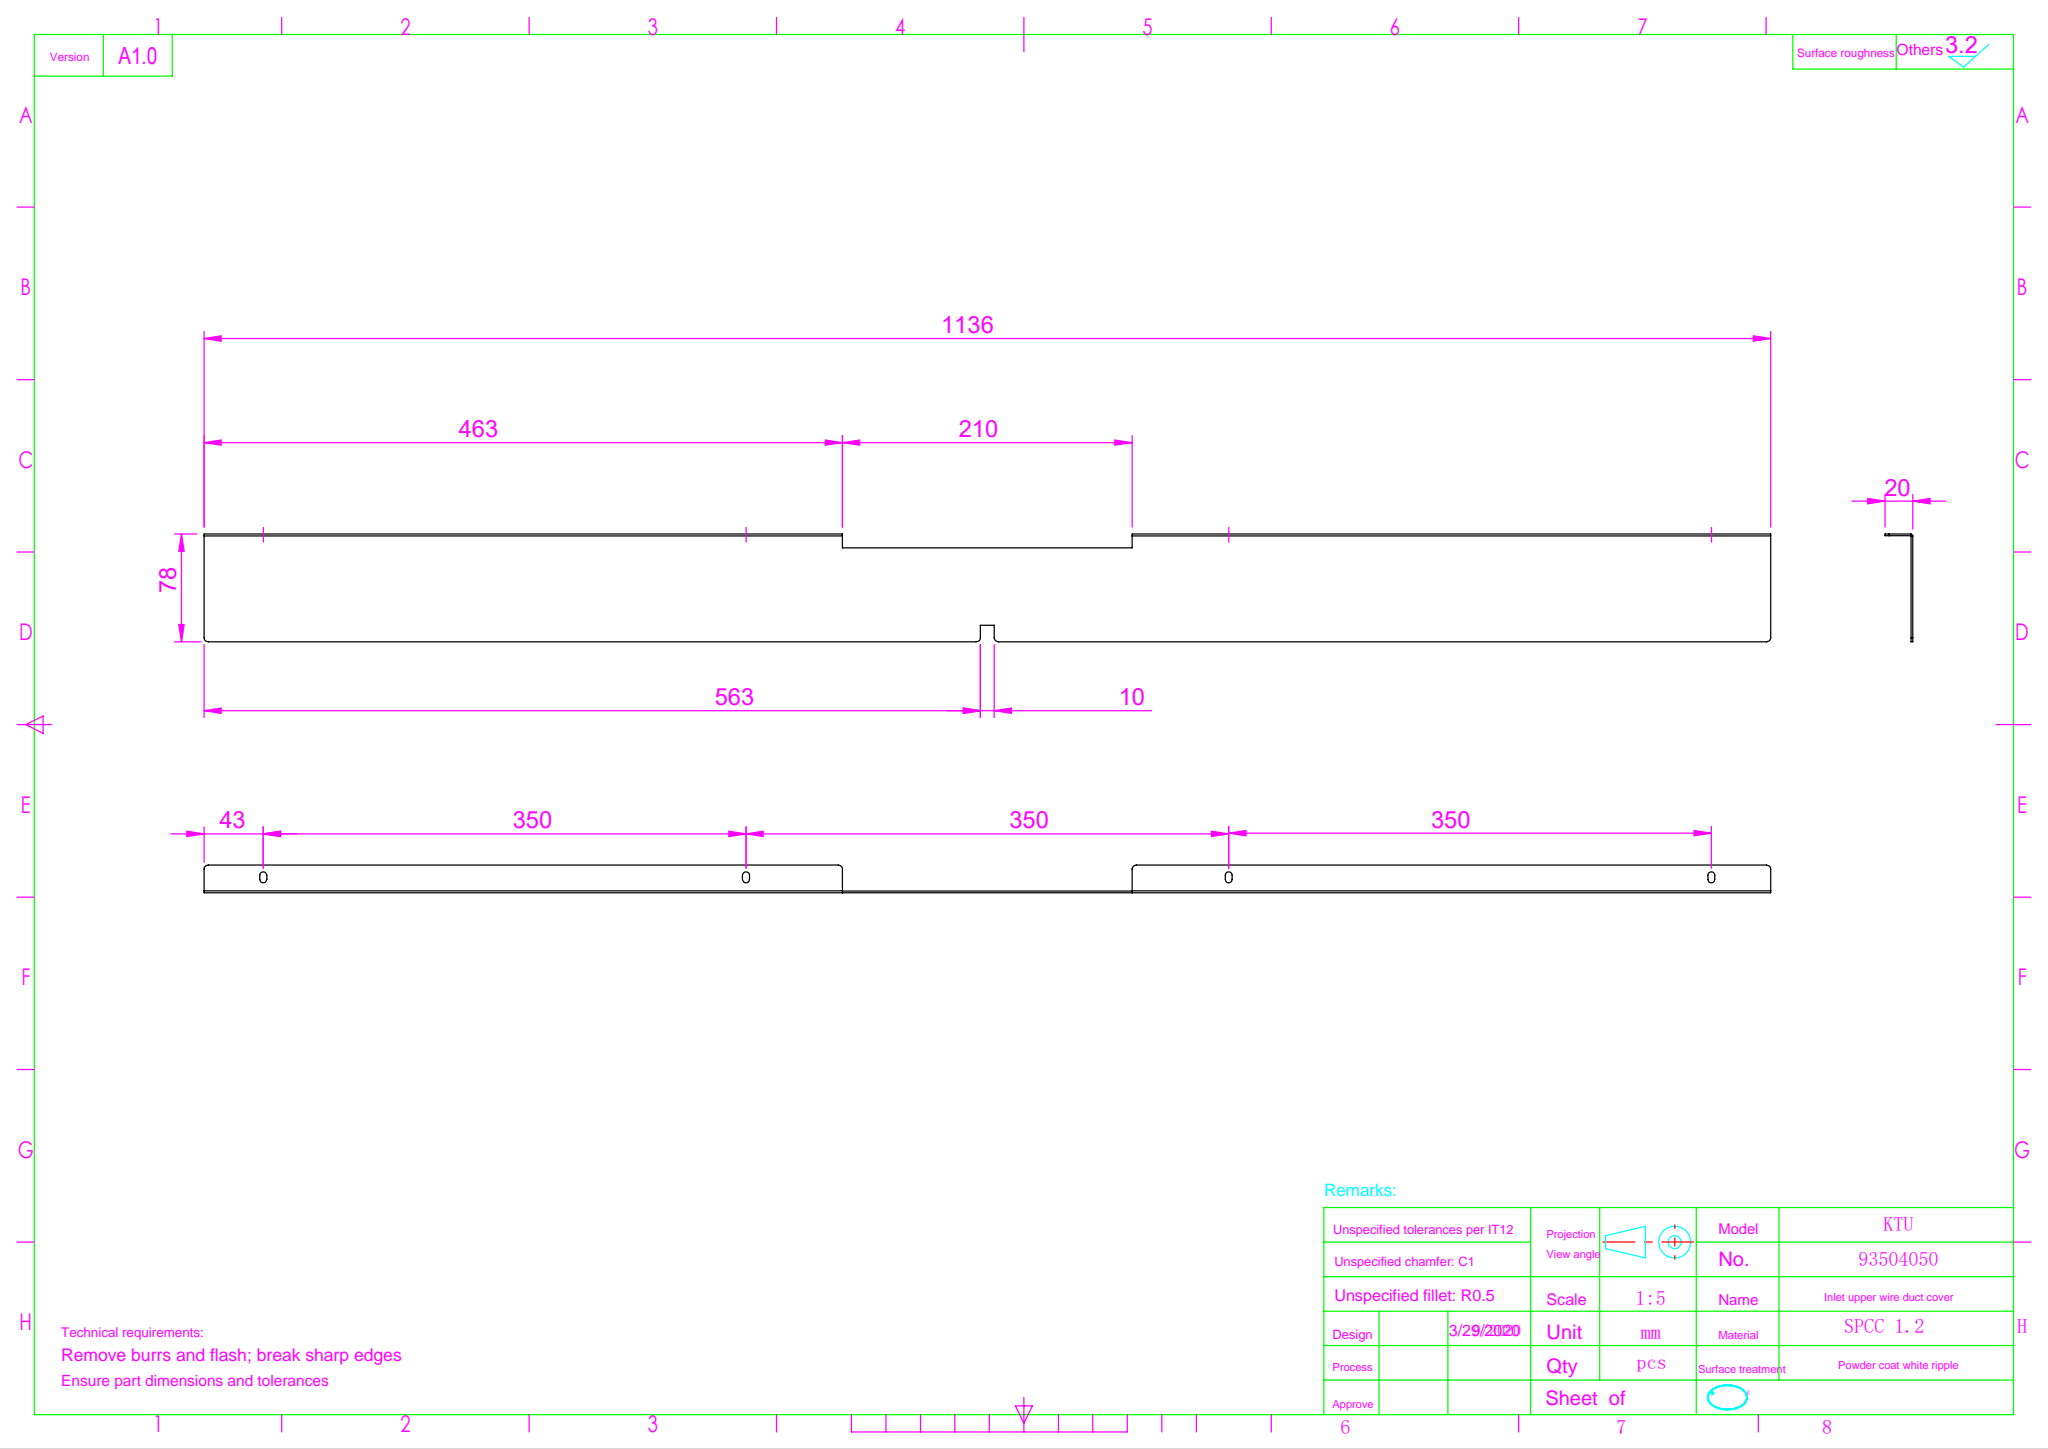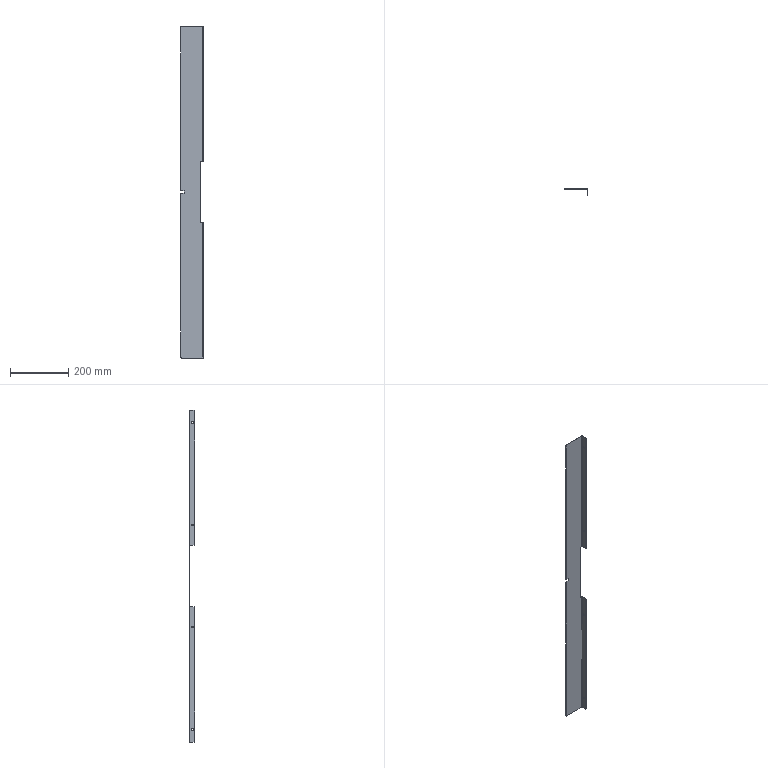Part | SolidWorks | features ICE 2, Fillet 1, FlatPattern 1, LPattern 1, SMBaseFlange 1, SheetMetal 1 | 1 solid | 50 faces | box 78 x 20 x 1136 mm | volume 123990 mm3 | plane 30 | cylinder 20 | commonest cylinder face diameters 5 x8 6 x8 0.4 x2 2.8 x2